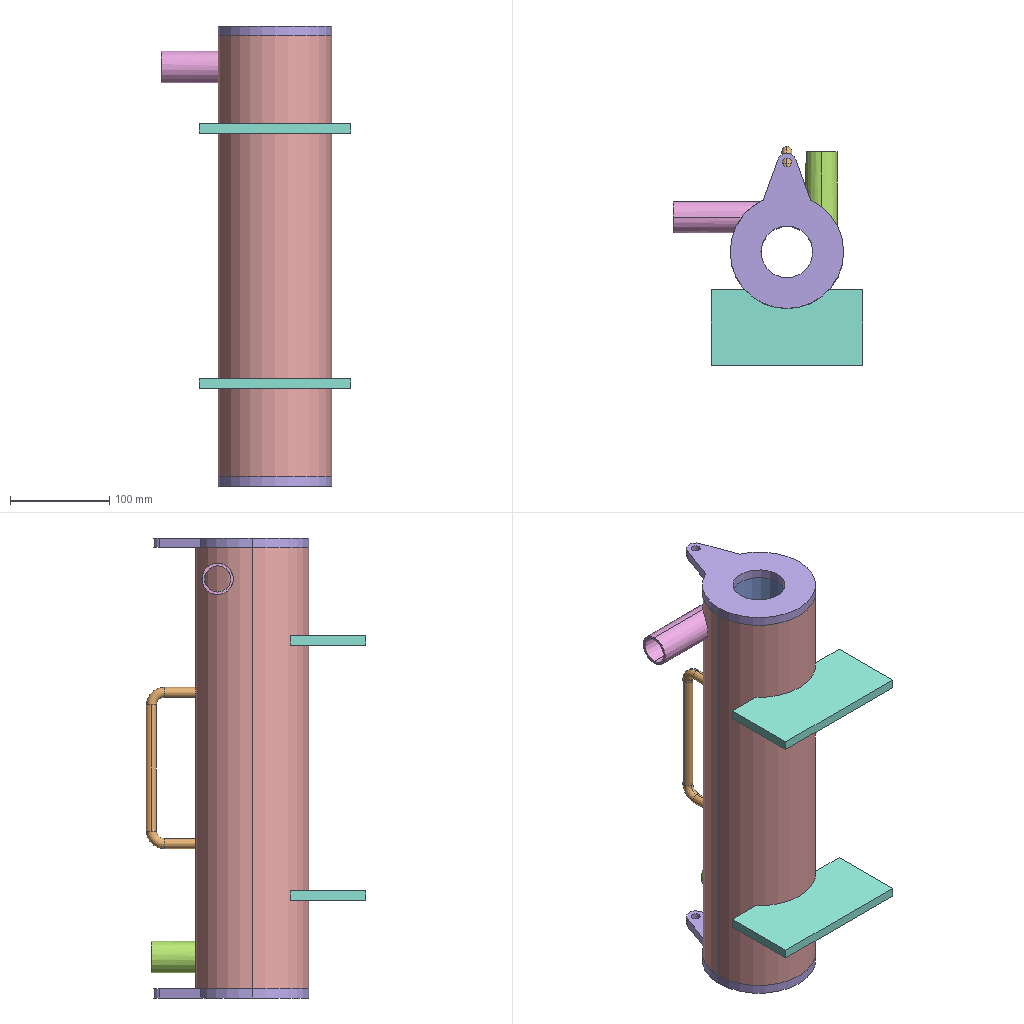Assembly | SolidWorks | 10 different items | 12 placed | box 190 x 221 x 464 mm
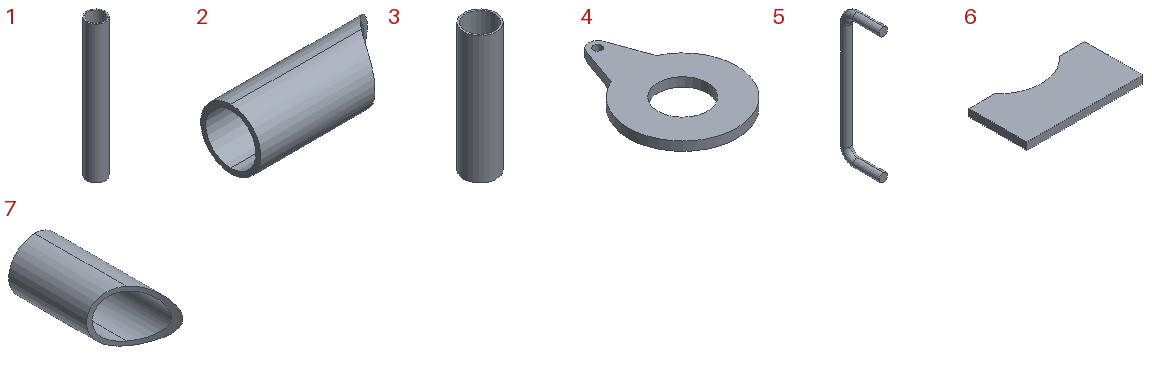Parts list (item | name | quantity | size | volume | features):
1 | - | x1 | 60.325 x 60.325 x 444.5 mm | 308147 mm3 | features Extrusion 1
2 | - | x1 | 88.118 x 31.75 x 31.75 mm | 16665 mm3 | features Extrusion 1
3 | - | x1 | 114.3 x 114.3 x 444.5 mm | 910233 mm3 | features Extrusion 1
4 | - | x2 | 114.3 x 156.675 x 9.525 mm | 88657 mm3 | features Extrusion 1
5 | - | x1 | 10.16 x 49.53 x 162.56 mm | 18679 mm3 | features Sweep 1
6 | - | x2 | 152.4 x 76.2 x 9.525 mm | 99906 mm3 | features Extrusion 1
7 | - | x1 | 31.75 x 75.418 x 31.75 mm | 13690 mm3 | features Extrusion 1
8 | Adjustment Cover | x1 | - | - | -
9 | Mirrored Adjustment Cover | x1 | - | - | -
10 | Part12 | x1 | - | - | -